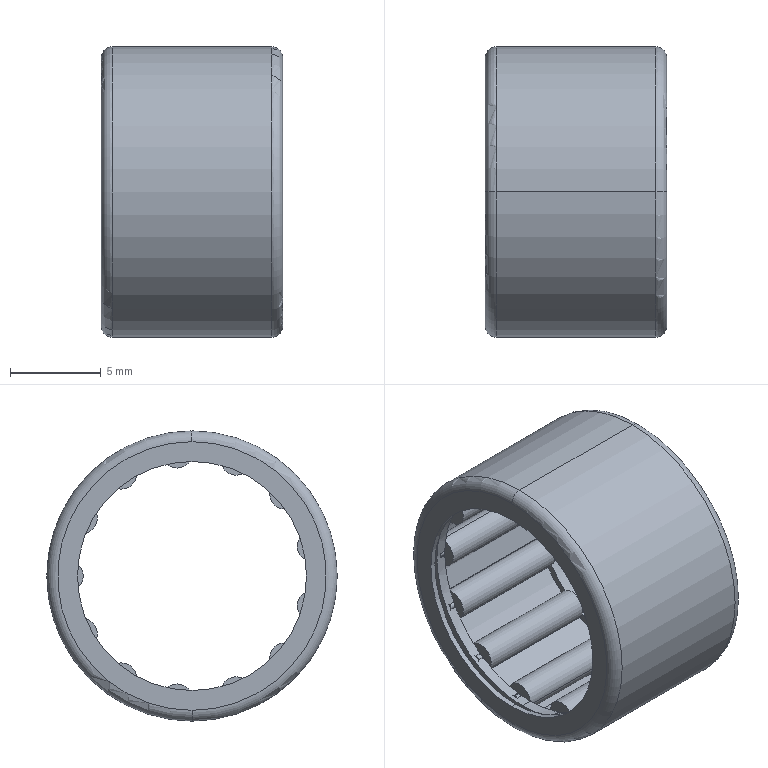Part | SolidWorks | features Revolution 3, CirPattern 2, MirrorPattern 2, Fillet 1, RevCut 1 | 1 solid | 221 faces | box 10 x 16 x 16 mm | volume 411.682 mm3 | cylinder 120 | plane 97 | torus 4 | commonest cylinder face diameters 0.475 x39 0.375 x26 1.69 x24 1.689 x15 12.625 x4 13.312 x4